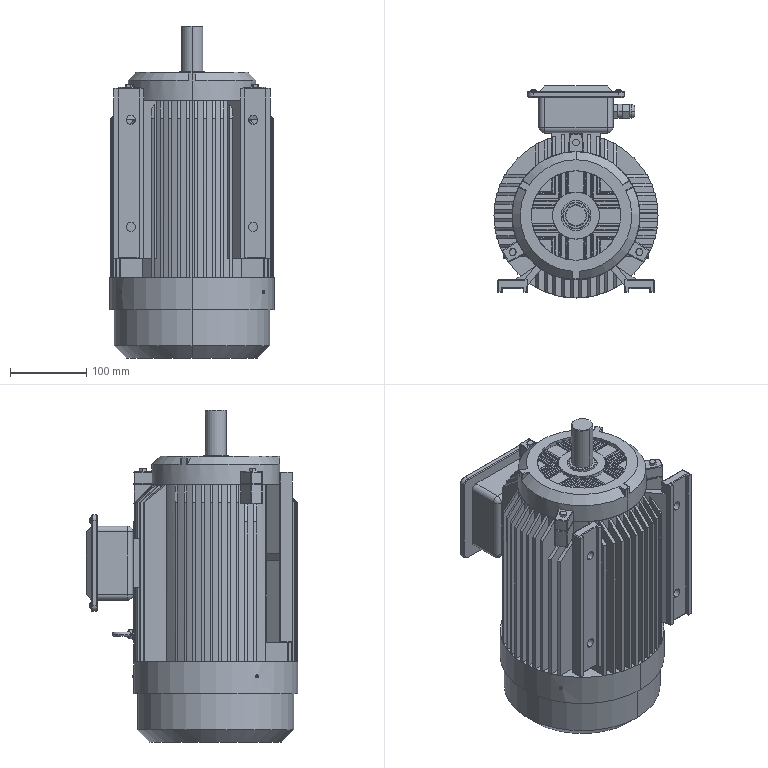Part | SolidWorks | features ICE 34, Fillet 14, CirPattern 7, Revolution 6, Chamfer 4, Extrusion 4, Dome 3, DeleteBody 2, RefAxis 2, MirrorPattern 1, MirrorSolid 1, MoveCopyBody 1, RevCut 1 | 2 solids | 890 faces | box 215 x 277.5 x 435 mm | volume 11674119 mm3 | plane 453 | cylinder 255 | cone 77 | sphere 52 | torus 45 | spline 8 | commonest cylinder face diameters 2 x124 215 x48 14.555 x12 2.175 x8 7.277 x8 12 x8